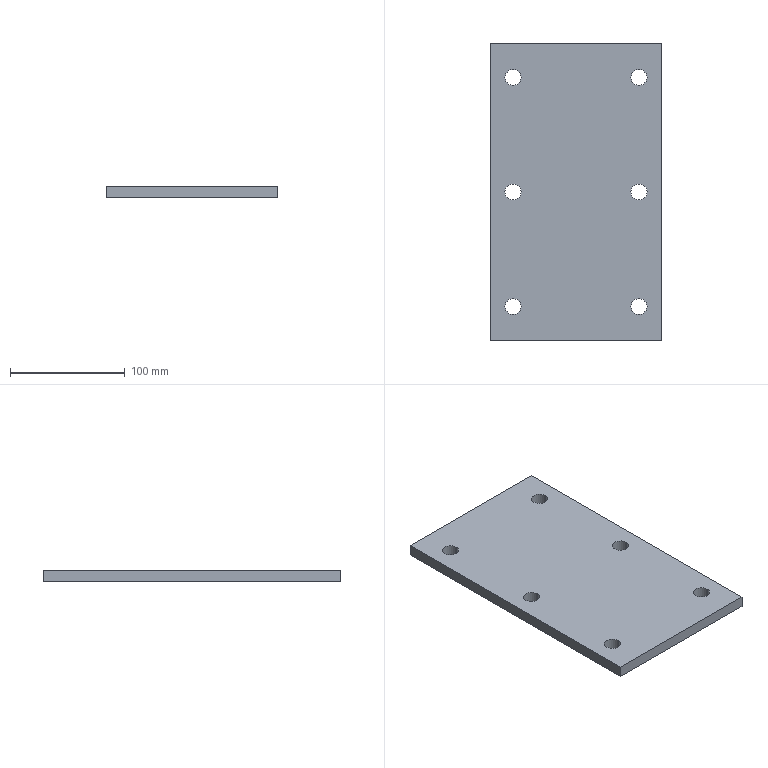Part | SolidWorks | features Extrusion 1, HoleWzd 1 | 1 solid | 18 faces | box 150 x 260 x 10 mm | volume 380764 mm3 | cylinder 12 | plane 6 | commonest cylinder face diameters 14 x12
STEP:
#1=CARTESIAN_POINT('',(-62.,100.,0.));
#2=VERTEX_POINT('',#1);
#3=CARTESIAN_POINT('',(-48.,100.,0.));
#4=VERTEX_POINT('',#3);
#5=CARTESIAN_POINT('',(-55.,100.,0.));
#6=DIRECTION('',(0.,0.,1.));
#7=DIRECTION('',(1.,0.,0.));
#8=AXIS2_PLACEMENT_3D('',#5,#6,#7);
#9=CIRCLE('',#8,7.);
#10=EDGE_CURVE('',#2,#4,#9,.T.);
#11=ORIENTED_EDGE('',*,*,#10,.F.);
#12=CARTESIAN_POINT('',(-62.,100.,10.));
#13=VERTEX_POINT('',#12);
#14=CARTESIAN_POINT('',(-62.,100.,10.));
#15=DIRECTION('',(0.,0.,1.));
#16=VECTOR('',#15,1000.);
#17=LINE('',#14,#16);
#18=EDGE_CURVE('',#2,#13,#17,.T.);
#19=ORIENTED_EDGE('',*,*,#18,.T.);
#20=CARTESIAN_POINT('',(-48.,100.,10.));
#21=VERTEX_POINT('',#20);
#22=CARTESIAN_POINT('',(-55.,100.,10.));
#23=DIRECTION('',(0.,0.,1.));
#24=DIRECTION('',(1.,0.,0.));
#25=AXIS2_PLACEMENT_3D('',#22,#23,#24);
#26=CIRCLE('',#25,7.);
#27=EDGE_CURVE('',#13,#21,#26,.T.);
#28=ORIENTED_EDGE('',*,*,#27,.T.);
#29=CARTESIAN_POINT('',(-48.,100.,10.));
#30=DIRECTION('',(0.,0.,1.));
#31=VECTOR('',#30,1000.);
#32=LINE('',#29,#31);
#33=EDGE_CURVE('',#4,#21,#32,.T.);
#34=ORIENTED_EDGE('',*,*,#33,.F.);
#35=EDGE_LOOP('',(#11,#19,#28,#34));
#36=FACE_OUTER_BOUND('',#35,.T.);
#37=CARTESIAN_POINT('',(-55.,100.,10.));
#38=DIRECTION('',(0.,0.,1.));
#39=DIRECTION('',(1.,0.,0.));
#40=AXIS2_PLACEMENT_3D('',#37,#38,#39);
#41=CYLINDRICAL_SURFACE('',#40,7.);
#42=ADVANCED_FACE('',(#36),#41,.F.);
#43=CARTESIAN_POINT('',(-62.,0.,0.));
#44=VERTEX_POINT('',#43);
#45=CARTESIAN_POINT('',(-48.,0.,0.));
#46=VERTEX_POINT('',#45);
#47=CARTESIAN_POINT('',(-55.,0.,0.));
#48=DIRECTION('',(0.,0.,1.));
#49=DIRECTION('',(1.,0.,0.));
#50=AXIS2_PLACEMENT_3D('',#47,#48,#49);
#51=CIRCLE('',#50,7.);
#52=EDGE_CURVE('',#44,#46,#51,.T.);
#53=ORIENTED_EDGE('',*,*,#52,.F.);
#54=CARTESIAN_POINT('',(-62.,0.,10.));
#55=VERTEX_POINT('',#54);
#56=CARTESIAN_POINT('',(-62.,0.,10.));
#57=DIRECTION('',(0.,0.,1.));
#58=VECTOR('',#57,1000.);
#59=LINE('',#56,#58);
#60=EDGE_CURVE('',#44,#55,#59,.T.);
#61=ORIENTED_EDGE('',*,*,#60,.T.);
#62=CARTESIAN_POINT('',(-48.,0.,10.));
#63=VERTEX_POINT('',#62);
#64=CARTESIAN_POINT('',(-55.,0.,10.));
#65=DIRECTION('',(0.,0.,1.));
#66=DIRECTION('',(1.,0.,0.));
#67=AXIS2_PLACEMENT_3D('',#64,#65,#66);
#68=CIRCLE('',#67,7.);
#69=EDGE_CURVE('',#55,#63,#68,.T.);
#70=ORIENTED_EDGE('',*,*,#69,.T.);
#71=CARTESIAN_POINT('',(-48.,0.,10.));
#72=DIRECTION('',(0.,0.,1.));
#73=VECTOR('',#72,1000.);
#74=LINE('',#71,#73);
#75=EDGE_CURVE('',#46,#63,#74,.T.);
#76=ORIENTED_EDGE('',*,*,#75,.F.);
#77=EDGE_LOOP('',(#53,#61,#70,#76));
#78=FACE_OUTER_BOUND('',#77,.T.);
#79=CARTESIAN_POINT('',(-55.,0.,10.));
#80=DIRECTION('',(0.,0.,1.));
#81=DIRECTION('',(1.,0.,0.));
#82=AXIS2_PLACEMENT_3D('',#79,#80,#81);
#83=CYLINDRICAL_SURFACE('',#82,7.);
#84=ADVANCED_FACE('',(#78),#83,.F.);
#85=CARTESIAN_POINT('',(-62.,-100.,0.));
#86=VERTEX_POINT('',#85);
#87=CARTESIAN_POINT('',(-48.,-100.,0.));
#88=VERTEX_POINT('',#87);
#89=CARTESIAN_POINT('',(-55.,-100.,0.));
#90=DIRECTION('',(0.,0.,1.));
#91=DIRECTION('',(1.,0.,0.));
#92=AXIS2_PLACEMENT_3D('',#89,#90,#91);
#93=CIRCLE('',#92,7.);
#94=EDGE_CURVE('',#86,#88,#93,.T.);
#95=ORIENTED_EDGE('',*,*,#94,.F.);
#96=CARTESIAN_POINT('',(-62.,-100.,10.));
#97=VERTEX_POINT('',#96);
#98=CARTESIAN_POINT('',(-62.,-100.,10.));
#99=DIRECTION('',(0.,0.,1.));
#100=VECTOR('',#99,1000.);
#101=LINE('',#98,#100);
#102=EDGE_CURVE('',#86,#97,#101,.T.);
#103=ORIENTED_EDGE('',*,*,#102,.T.);
#104=CARTESIAN_POINT('',(-48.,-100.,10.));
#105=VERTEX_POINT('',#104);
#106=CARTESIAN_POINT('',(-55.,-100.,10.));
#107=DIRECTION('',(0.,0.,1.));
#108=DIRECTION('',(1.,0.,0.));
#109=AXIS2_PLACEMENT_3D('',#106,#107,#108);
#110=CIRCLE('',#109,7.);
#111=EDGE_CURVE('',#97,#105,#110,.T.);
#112=ORIENTED_EDGE('',*,*,#111,.T.);
#113=CARTESIAN_POINT('',(-48.,-100.,10.));
#114=DIRECTION('',(0.,0.,1.));
#115=VECTOR('',#114,1000.);
#116=LINE('',#113,#115);
#117=EDGE_CURVE('',#88,#105,#116,.T.);
#118=ORIENTED_EDGE('',*,*,#117,.F.);
#119=EDGE_LOOP('',(#95,#103,#112,#118));
#120=FACE_OUTER_BOUND('',#119,.T.);
#121=CARTESIAN_POINT('',(-55.,-100.,10.));
#122=DIRECTION('',(0.,0.,1.));
#123=DIRECTION('',(1.,0.,0.));
#124=AXIS2_PLACEMENT_3D('',#121,#122,#123);
#125=CYLINDRICAL_SURFACE('',#124,7.);
#126=ADVANCED_FACE('',(#120),#125,.F.);
#127=CARTESIAN_POINT('',(48.,-100.,0.));
#128=VERTEX_POINT('',#127);
#129=CARTESIAN_POINT('',(62.,-100.,0.));
#130=VERTEX_POINT('',#129);
#131=CARTESIAN_POINT('',(55.,-100.,0.));
#132=DIRECTION('',(0.,0.,1.));
#133=DIRECTION('',(1.,0.,0.));
#134=AXIS2_PLACEMENT_3D('',#131,#132,#133);
#135=CIRCLE('',#134,7.);
#136=EDGE_CURVE('',#128,#130,#135,.T.);
#137=ORIENTED_EDGE('',*,*,#136,.F.);
#138=CARTESIAN_POINT('',(48.,-100.,10.));
#139=VERTEX_POINT('',#138);
#140=CARTESIAN_POINT('',(48.,-100.,10.));
#141=DIRECTION('',(0.,0.,1.));
#142=VECTOR('',#141,1000.);
#143=LINE('',#140,#142);
#144=EDGE_CURVE('',#128,#139,#143,.T.);
#145=ORIENTED_EDGE('',*,*,#144,.T.);
#146=CARTESIAN_POINT('',(62.,-100.,10.));
#147=VERTEX_POINT('',#146);
#148=CARTESIAN_POINT('',(55.,-100.,10.));
#149=DIRECTION('',(0.,0.,1.));
#150=DIRECTION('',(1.,0.,0.));
#151=AXIS2_PLACEMENT_3D('',#148,#149,#150);
#152=CIRCLE('',#151,7.);
#153=EDGE_CURVE('',#139,#147,#152,.T.);
#154=ORIENTED_EDGE('',*,*,#153,.T.);
#155=CARTESIAN_POINT('',(62.,-100.,10.));
#156=DIRECTION('',(0.,0.,1.));
#157=VECTOR('',#156,1000.);
#158=LINE('',#155,#157);
#159=EDGE_CURVE('',#130,#147,#158,.T.);
#160=ORIENTED_EDGE('',*,*,#159,.F.);
#161=EDGE_LOOP('',(#137,#145,#154,#160));
#162=FACE_OUTER_BOUND('',#161,.T.);
#163=CARTESIAN_POINT('',(55.,-100.,10.));
#164=DIRECTION('',(0.,0.,1.));
#165=DIRECTION('',(1.,0.,0.));
#166=AXIS2_PLACEMENT_3D('',#163,#164,#165);
#167=CYLINDRICAL_SURFACE('',#166,7.);
#168=ADVANCED_FACE('',(#162),#167,.F.);
#169=CARTESIAN_POINT('',(48.,0.,0.));
#170=VERTEX_POINT('',#169);
#171=CARTESIAN_POINT('',(62.,0.,0.));
#172=VERTEX_POINT('',#171);
#173=CARTESIAN_POINT('',(55.,0.,0.));
#174=DIRECTION('',(0.,0.,1.));
#175=DIRECTION('',(1.,0.,0.));
#176=AXIS2_PLACEMENT_3D('',#173,#174,#175);
#177=CIRCLE('',#176,7.);
#178=EDGE_CURVE('',#170,#172,#177,.T.);
#179=ORIENTED_EDGE('',*,*,#178,.F.);
#180=CARTESIAN_POINT('',(48.,0.,10.));
#181=VERTEX_POINT('',#180);
#182=CARTESIAN_POINT('',(48.,0.,10.));
#183=DIRECTION('',(0.,0.,1.));
#184=VECTOR('',#183,1000.);
#185=LINE('',#182,#184);
#186=EDGE_CURVE('',#170,#181,#185,.T.);
#187=ORIENTED_EDGE('',*,*,#186,.T.);
#188=CARTESIAN_POINT('',(62.,0.,10.));
#189=VERTEX_POINT('',#188);
#190=CARTESIAN_POINT('',(55.,0.,10.));
#191=DIRECTION('',(0.,0.,1.));
#192=DIRECTION('',(1.,0.,0.));
#193=AXIS2_PLACEMENT_3D('',#190,#191,#192);
#194=CIRCLE('',#193,7.);
#195=EDGE_CURVE('',#181,#189,#194,.T.);
#196=ORIENTED_EDGE('',*,*,#195,.T.);
#197=CARTESIAN_POINT('',(62.,0.,10.));
#198=DIRECTION('',(0.,0.,1.));
#199=VECTOR('',#198,1000.);
#200=LINE('',#197,#199);
#201=EDGE_CURVE('',#172,#189,#200,.T.);
#202=ORIENTED_EDGE('',*,*,#201,.F.);
#203=EDGE_LOOP('',(#179,#187,#196,#202));
#204=FACE_OUTER_BOUND('',#203,.T.);
#205=CARTESIAN_POINT('',(55.,0.,10.));
#206=DIRECTION('',(0.,0.,1.));
#207=DIRECTION('',(1.,0.,0.));
#208=AXIS2_PLACEMENT_3D('',#205,#206,#207);
#209=CYLINDRICAL_SURFACE('',#208,7.);
#210=ADVANCED_FACE('',(#204),#209,.F.);
#211=CARTESIAN_POINT('',(48.,100.,0.));
#212=VERTEX_POINT('',#211);
#213=CARTESIAN_POINT('',(62.,100.,0.));
#214=VERTEX_POINT('',#213);
#215=CARTESIAN_POINT('',(55.,100.,0.));
#216=DIRECTION('',(0.,0.,1.));
#217=DIRECTION('',(1.,0.,0.));
#218=AXIS2_PLACEMENT_3D('',#215,#216,#217);
#219=CIRCLE('',#218,7.);
#220=EDGE_CURVE('',#212,#214,#219,.T.);
#221=ORIENTED_EDGE('',*,*,#220,.F.);
#222=CARTESIAN_POINT('',(48.,100.,10.));
#223=VERTEX_POINT('',#222);
#224=CARTESIAN_POINT('',(48.,100.,10.));
#225=DIRECTION('',(0.,0.,1.));
#226=VECTOR('',#225,1000.);
#227=LINE('',#224,#226);
#228=EDGE_CURVE('',#212,#223,#227,.T.);
#229=ORIENTED_EDGE('',*,*,#228,.T.);
#230=CARTESIAN_POINT('',(62.,100.,10.));
#231=VERTEX_POINT('',#230);
#232=CARTESIAN_POINT('',(55.,100.,10.));
#233=DIRECTION('',(0.,0.,1.));
#234=DIRECTION('',(1.,0.,0.));
#235=AXIS2_PLACEMENT_3D('',#232,#233,#234);
#236=CIRCLE('',#235,7.);
#237=EDGE_CURVE('',#223,#231,#236,.T.);
#238=ORIENTED_EDGE('',*,*,#237,.T.);
#239=CARTESIAN_POINT('',(62.,100.,10.));
#240=DIRECTION('',(0.,0.,1.));
#241=VECTOR('',#240,1000.);
#242=LINE('',#239,#241);
#243=EDGE_CURVE('',#214,#231,#242,.T.);
#244=ORIENTED_EDGE('',*,*,#243,.F.);
#245=EDGE_LOOP('',(#221,#229,#238,#244));
#246=FACE_OUTER_BOUND('',#245,.T.);
#247=CARTESIAN_POINT('',(55.,100.,10.));
#248=DIRECTION('',(0.,0.,1.));
#249=DIRECTION('',(1.,0.,0.));
#250=AXIS2_PLACEMENT_3D('',#247,#248,#249);
#251=CYLINDRICAL_SURFACE('',#250,7.);
#252=ADVANCED_FACE('',(#246),#251,.F.);
#253=CARTESIAN_POINT('',(-75.,130.,0.));
#254=VERTEX_POINT('',#253);
#255=CARTESIAN_POINT('',(-75.,-130.,0.));
#256=VERTEX_POINT('',#255);
#257=CARTESIAN_POINT('',(-75.,-130.,0.));
#258=DIRECTION('',(0.,-1.,0.));
#259=VECTOR('',#258,1000.);
#260=LINE('',#257,#259);
#261=EDGE_CURVE('',#254,#256,#260,.T.);
#262=ORIENTED_EDGE('',*,*,#261,.T.);
#263=CARTESIAN_POINT('',(-75.,-130.,10.));
#264=VERTEX_POINT('',#263);
#265=CARTESIAN_POINT('',(-75.,-130.,10.));
#266=DIRECTION('',(0.,0.,-1.));
#267=VECTOR('',#266,1000.);
#268=LINE('',#265,#267);
#269=EDGE_CURVE('',#264,#256,#268,.T.);
#270=ORIENTED_EDGE('',*,*,#269,.F.);
#271=CARTESIAN_POINT('',(-75.,130.,10.));
#272=VERTEX_POINT('',#271);
#273=CARTESIAN_POINT('',(-75.,-130.,10.));
#274=DIRECTION('',(0.,-1.,0.));
#275=VECTOR('',#274,1000.);
#276=LINE('',#273,#275);
#277=EDGE_CURVE('',#272,#264,#276,.T.);
#278=ORIENTED_EDGE('',*,*,#277,.F.);
#279=CARTESIAN_POINT('',(-75.,130.,10.));
#280=DIRECTION('',(0.,0.,-1.));
#281=VECTOR('',#280,1000.);
#282=LINE('',#279,#281);
#283=EDGE_CURVE('',#272,#254,#282,.T.);
#284=ORIENTED_EDGE('',*,*,#283,.T.);
#285=EDGE_LOOP('',(#262,#270,#278,#284));
#286=FACE_OUTER_BOUND('',#285,.T.);
#287=CARTESIAN_POINT('',(-75.,-130.,10.));
#288=DIRECTION('',(1.,0.,0.));
#289=DIRECTION('',(0.,0.,-1.));
#290=AXIS2_PLACEMENT_3D('',#287,#288,#289);
#291=PLANE('',#290);
#292=ADVANCED_FACE('',(#286),#291,.F.);
#293=CARTESIAN_POINT('',(75.,-130.,0.));
#294=VERTEX_POINT('',#293);
#295=CARTESIAN_POINT('',(75.,-130.,0.));
#296=DIRECTION('',(1.,0.,0.));
#297=VECTOR('',#296,1000.);
#298=LINE('',#295,#297);
#299=EDGE_CURVE('',#256,#294,#298,.T.);
#300=ORIENTED_EDGE('',*,*,#299,.T.);
#301=CARTESIAN_POINT('',(75.,-130.,10.));
#302=VERTEX_POINT('',#301);
#303=CARTESIAN_POINT('',(75.,-130.,10.));
#304=DIRECTION('',(0.,0.,-1.));
#305=VECTOR('',#304,1000.);
#306=LINE('',#303,#305);
#307=EDGE_CURVE('',#302,#294,#306,.T.);
#308=ORIENTED_EDGE('',*,*,#307,.F.);
#309=CARTESIAN_POINT('',(75.,-130.,10.));
#310=DIRECTION('',(1.,0.,0.));
#311=VECTOR('',#310,1000.);
#312=LINE('',#309,#311);
#313=EDGE_CURVE('',#264,#302,#312,.T.);
#314=ORIENTED_EDGE('',*,*,#313,.F.);
#315=ORIENTED_EDGE('',*,*,#269,.T.);
#316=EDGE_LOOP('',(#300,#308,#314,#315));
#317=FACE_OUTER_BOUND('',#316,.T.);
#318=CARTESIAN_POINT('',(75.,-130.,10.));
#319=DIRECTION('',(0.,1.,0.));
#320=DIRECTION('',(-1.,0.,0.));
#321=AXIS2_PLACEMENT_3D('',#318,#319,#320);
#322=PLANE('',#321);
#323=ADVANCED_FACE('',(#317),#322,.F.);
#324=CARTESIAN_POINT('',(75.,130.,0.));
#325=VERTEX_POINT('',#324);
#326=CARTESIAN_POINT('',(75.,-130.,0.));
#327=DIRECTION('',(0.,1.,0.));
#328=VECTOR('',#327,1000.);
#329=LINE('',#326,#328);
#330=EDGE_CURVE('',#294,#325,#329,.T.);
#331=ORIENTED_EDGE('',*,*,#330,.T.);
#332=CARTESIAN_POINT('',(75.,130.,10.));
#333=VERTEX_POINT('',#332);
#334=CARTESIAN_POINT('',(75.,130.,10.));
#335=DIRECTION('',(0.,0.,-1.));
#336=VECTOR('',#335,1000.);
#337=LINE('',#334,#336);
#338=EDGE_CURVE('',#333,#325,#337,.T.);
#339=ORIENTED_EDGE('',*,*,#338,.F.);
#340=CARTESIAN_POINT('',(75.,-130.,10.));
#341=DIRECTION('',(0.,1.,0.));
#342=VECTOR('',#341,1000.);
#343=LINE('',#340,#342);
#344=EDGE_CURVE('',#302,#333,#343,.T.);
#345=ORIENTED_EDGE('',*,*,#344,.F.);
#346=ORIENTED_EDGE('',*,*,#307,.T.);
#347=EDGE_LOOP('',(#331,#339,#345,#346));
#348=FACE_OUTER_BOUND('',#347,.T.);
#349=CARTESIAN_POINT('',(75.,-130.,10.));
#350=DIRECTION('',(-1.,0.,0.));
#351=DIRECTION('',(0.,0.,1.));
#352=AXIS2_PLACEMENT_3D('',#349,#350,#351);
#353=PLANE('',#352);
#354=ADVANCED_FACE('',(#348),#353,.F.);
#355=CARTESIAN_POINT('',(75.,130.,0.));
#356=DIRECTION('',(-1.,0.,0.));
#357=VECTOR('',#356,1000.);
#358=LINE('',#355,#357);
#359=EDGE_CURVE('',#325,#254,#358,.T.);
#360=ORIENTED_EDGE('',*,*,#359,.T.);
#361=ORIENTED_EDGE('',*,*,#283,.F.);
#362=CARTESIAN_POINT('',(75.,130.,10.));
#363=DIRECTION('',(-1.,0.,0.));
#364=VECTOR('',#363,1000.);
#365=LINE('',#362,#364);
#366=EDGE_CURVE('',#333,#272,#365,.T.);
#367=ORIENTED_EDGE('',*,*,#366,.F.);
#368=ORIENTED_EDGE('',*,*,#338,.T.);
#369=EDGE_LOOP('',(#360,#361,#367,#368));
#370=FACE_OUTER_BOUND('',#369,.T.);
#371=CARTESIAN_POINT('',(75.,130.,10.));
#372=DIRECTION('',(0.,-1.,0.));
#373=DIRECTION('',(0.,0.,-1.));
#374=AXIS2_PLACEMENT_3D('',#371,#372,#373);
#375=PLANE('',#374);
#376=ADVANCED_FACE('',(#370),#375,.F.);
#377=CARTESIAN_POINT('',(-55.,100.,10.));
#378=DIRECTION('',(0.,0.,1.));
#379=DIRECTION('',(1.,0.,0.));
#380=AXIS2_PLACEMENT_3D('',#377,#378,#379);
#381=CIRCLE('',#380,7.);
#382=EDGE_CURVE('',#21,#13,#381,.T.);
#383=ORIENTED_EDGE('',*,*,#382,.F.);
#384=ORIENTED_EDGE('',*,*,#27,.F.);
#385=EDGE_LOOP('',(#383,#384));
#386=FACE_BOUND('',#385,.T.);
#387=CARTESIAN_POINT('',(-55.,0.,10.));
#388=DIRECTION('',(0.,0.,1.));
#389=DIRECTION('',(1.,0.,0.));
#390=AXIS2_PLACEMENT_3D('',#387,#388,#389);
#391=CIRCLE('',#390,7.);
#392=EDGE_CURVE('',#63,#55,#391,.T.);
#393=ORIENTED_EDGE('',*,*,#392,.F.);
#394=ORIENTED_EDGE('',*,*,#69,.F.);
#395=EDGE_LOOP('',(#393,#394));
#396=FACE_BOUND('',#395,.T.);
#397=CARTESIAN_POINT('',(-55.,-100.,10.));
#398=DIRECTION('',(0.,0.,1.));
#399=DIRECTION('',(1.,0.,0.));
#400=AXIS2_PLACEMENT_3D('',#397,#398,#399);
#401=CIRCLE('',#400,7.);
#402=EDGE_CURVE('',#105,#97,#401,.T.);
#403=ORIENTED_EDGE('',*,*,#402,.F.);
#404=ORIENTED_EDGE('',*,*,#111,.F.);
#405=EDGE_LOOP('',(#403,#404));
#406=FACE_BOUND('',#405,.T.);
#407=CARTESIAN_POINT('',(55.,-100.,10.));
#408=DIRECTION('',(0.,0.,1.));
#409=DIRECTION('',(1.,0.,0.));
#410=AXIS2_PLACEMENT_3D('',#407,#408,#409);
#411=CIRCLE('',#410,7.);
#412=EDGE_CURVE('',#147,#139,#411,.T.);
#413=ORIENTED_EDGE('',*,*,#412,.F.);
#414=ORIENTED_EDGE('',*,*,#153,.F.);
#415=EDGE_LOOP('',(#413,#414));
#416=FACE_BOUND('',#415,.T.);
#417=CARTESIAN_POINT('',(55.,0.,10.));
#418=DIRECTION('',(0.,0.,1.));
#419=DIRECTION('',(1.,0.,0.));
#420=AXIS2_PLACEMENT_3D('',#417,#418,#419);
#421=CIRCLE('',#420,7.);
#422=EDGE_CURVE('',#189,#181,#421,.T.);
#423=ORIENTED_EDGE('',*,*,#422,.F.);
#424=ORIENTED_EDGE('',*,*,#195,.F.);
#425=EDGE_LOOP('',(#423,#424));
#426=FACE_BOUND('',#425,.T.);
#427=CARTESIAN_POINT('',(55.,100.,10.));
#428=DIRECTION('',(0.,0.,1.));
#429=DIRECTION('',(1.,0.,0.));
#430=AXIS2_PLACEMENT_3D('',#427,#428,#429);
#431=CIRCLE('',#430,7.);
#432=EDGE_CURVE('',#231,#223,#431,.T.);
#433=ORIENTED_EDGE('',*,*,#432,.F.);
#434=ORIENTED_EDGE('',*,*,#237,.F.);
#435=EDGE_LOOP('',(#433,#434));
#436=FACE_BOUND('',#435,.T.);
#437=ORIENTED_EDGE('',*,*,#277,.T.);
#438=ORIENTED_EDGE('',*,*,#313,.T.);
#439=ORIENTED_EDGE('',*,*,#344,.T.);
#440=ORIENTED_EDGE('',*,*,#366,.T.);
#441=EDGE_LOOP('',(#437,#438,#439,#440));
#442=FACE_OUTER_BOUND('',#441,.T.);
#443=CARTESIAN_POINT('',(0.,0.,10.));
#444=DIRECTION('',(0.,0.,1.));
#445=DIRECTION('',(1.,0.,0.));
#446=AXIS2_PLACEMENT_3D('',#443,#444,#445);
#447=PLANE('',#446);
#448=ADVANCED_FACE('',(#386,#396,#406,#416,#426,#436,#442),#447,.T.);
#449=CARTESIAN_POINT('',(-55.,100.,0.));
#450=DIRECTION('',(0.,0.,1.));
#451=DIRECTION('',(1.,0.,0.));
#452=AXIS2_PLACEMENT_3D('',#449,#450,#451);
#453=CIRCLE('',#452,7.);
#454=EDGE_CURVE('',#4,#2,#453,.T.);
#455=ORIENTED_EDGE('',*,*,#454,.T.);
#456=ORIENTED_EDGE('',*,*,#10,.T.);
#457=EDGE_LOOP('',(#455,#456));
#458=FACE_BOUND('',#457,.T.);
#459=CARTESIAN_POINT('',(-55.,0.,0.));
#460=DIRECTION('',(0.,0.,1.));
#461=DIRECTION('',(1.,0.,0.));
#462=AXIS2_PLACEMENT_3D('',#459,#460,#461);
#463=CIRCLE('',#462,7.);
#464=EDGE_CURVE('',#46,#44,#463,.T.);
#465=ORIENTED_EDGE('',*,*,#464,.T.);
#466=ORIENTED_EDGE('',*,*,#52,.T.);
#467=EDGE_LOOP('',(#465,#466));
#468=FACE_BOUND('',#467,.T.);
#469=CARTESIAN_POINT('',(-55.,-100.,0.));
#470=DIRECTION('',(0.,0.,1.));
#471=DIRECTION('',(1.,0.,0.));
#472=AXIS2_PLACEMENT_3D('',#469,#470,#471);
#473=CIRCLE('',#472,7.);
#474=EDGE_CURVE('',#88,#86,#473,.T.);
#475=ORIENTED_EDGE('',*,*,#474,.T.);
#476=ORIENTED_EDGE('',*,*,#94,.T.);
#477=EDGE_LOOP('',(#475,#476));
#478=FACE_BOUND('',#477,.T.);
#479=CARTESIAN_POINT('',(55.,-100.,0.));
#480=DIRECTION('',(0.,0.,1.));
#481=DIRECTION('',(1.,0.,0.));
#482=AXIS2_PLACEMENT_3D('',#479,#480,#481);
#483=CIRCLE('',#482,7.);
#484=EDGE_CURVE('',#130,#128,#483,.T.);
#485=ORIENTED_EDGE('',*,*,#484,.T.);
#486=ORIENTED_EDGE('',*,*,#136,.T.);
#487=EDGE_LOOP('',(#485,#486));
#488=FACE_BOUND('',#487,.T.);
#489=CARTESIAN_POINT('',(55.,0.,0.));
#490=DIRECTION('',(0.,0.,1.));
#491=DIRECTION('',(1.,0.,0.));
#492=AXIS2_PLACEMENT_3D('',#489,#490,#491);
#493=CIRCLE('',#492,7.);
#494=EDGE_CURVE('',#172,#170,#493,.T.);
#495=ORIENTED_EDGE('',*,*,#494,.T.);
#496=ORIENTED_EDGE('',*,*,#178,.T.);
#497=EDGE_LOOP('',(#495,#496));
#498=FACE_BOUND('',#497,.T.);
#499=CARTESIAN_POINT('',(55.,100.,0.));
#500=DIRECTION('',(0.,0.,1.));
#501=DIRECTION('',(1.,0.,0.));
#502=AXIS2_PLACEMENT_3D('',#499,#500,#501);
#503=CIRCLE('',#502,7.);
#504=EDGE_CURVE('',#214,#212,#503,.T.);
#505=ORIENTED_EDGE('',*,*,#504,.T.);
#506=ORIENTED_EDGE('',*,*,#220,.T.);
#507=EDGE_LOOP('',(#505,#506));
#508=FACE_BOUND('',#507,.T.);
#509=ORIENTED_EDGE('',*,*,#261,.F.);
#510=ORIENTED_EDGE('',*,*,#359,.F.);
#511=ORIENTED_EDGE('',*,*,#330,.F.);
#512=ORIENTED_EDGE('',*,*,#299,.F.);
#513=EDGE_LOOP('',(#509,#510,#511,#512));
#514=FACE_OUTER_BOUND('',#513,.T.);
#515=CARTESIAN_POINT('',(0.,0.,0.));
#516=DIRECTION('',(0.,0.,1.));
#517=DIRECTION('',(1.,0.,0.));
#518=AXIS2_PLACEMENT_3D('',#515,#516,#517);
#519=PLANE('',#518);
#520=ADVANCED_FACE('',(#458,#468,#478,#488,#498,#508,#514),#519,.F.);
#521=ORIENTED_EDGE('',*,*,#228,.F.);
#522=ORIENTED_EDGE('',*,*,#504,.F.);
#523=ORIENTED_EDGE('',*,*,#243,.T.);
#524=ORIENTED_EDGE('',*,*,#432,.T.);
#525=EDGE_LOOP('',(#521,#522,#523,#524));
#526=FACE_OUTER_BOUND('',#525,.T.);
#527=CARTESIAN_POINT('',(55.,100.,10.));
#528=DIRECTION('',(0.,0.,1.));
#529=DIRECTION('',(1.,0.,0.));
#530=AXIS2_PLACEMENT_3D('',#527,#528,#529);
#531=CYLINDRICAL_SURFACE('',#530,7.);
#532=ADVANCED_FACE('',(#526),#531,.F.);
#533=ORIENTED_EDGE('',*,*,#186,.F.);
#534=ORIENTED_EDGE('',*,*,#494,.F.);
#535=ORIENTED_EDGE('',*,*,#201,.T.);
#536=ORIENTED_EDGE('',*,*,#422,.T.);
#537=EDGE_LOOP('',(#533,#534,#535,#536));
#538=FACE_OUTER_BOUND('',#537,.T.);
#539=CARTESIAN_POINT('',(55.,0.,10.));
#540=DIRECTION('',(0.,0.,1.));
#541=DIRECTION('',(1.,0.,0.));
#542=AXIS2_PLACEMENT_3D('',#539,#540,#541);
#543=CYLINDRICAL_SURFACE('',#542,7.);
#544=ADVANCED_FACE('',(#538),#543,.F.);
#545=ORIENTED_EDGE('',*,*,#144,.F.);
#546=ORIENTED_EDGE('',*,*,#484,.F.);
#547=ORIENTED_EDGE('',*,*,#159,.T.);
#548=ORIENTED_EDGE('',*,*,#412,.T.);
#549=EDGE_LOOP('',(#545,#546,#547,#548));
#550=FACE_OUTER_BOUND('',#549,.T.);
#551=CARTESIAN_POINT('',(55.,-100.,10.));
#552=DIRECTION('',(0.,0.,1.));
#553=DIRECTION('',(1.,0.,0.));
#554=AXIS2_PLACEMENT_3D('',#551,#552,#553);
#555=CYLINDRICAL_SURFACE('',#554,7.);
#556=ADVANCED_FACE('',(#550),#555,.F.);
#557=ORIENTED_EDGE('',*,*,#102,.F.);
#558=ORIENTED_EDGE('',*,*,#474,.F.);
#559=ORIENTED_EDGE('',*,*,#117,.T.);
#560=ORIENTED_EDGE('',*,*,#402,.T.);
#561=EDGE_LOOP('',(#557,#558,#559,#560));
#562=FACE_OUTER_BOUND('',#561,.T.);
#563=CARTESIAN_POINT('',(-55.,-100.,10.));
#564=DIRECTION('',(0.,0.,1.));
#565=DIRECTION('',(1.,0.,0.));
#566=AXIS2_PLACEMENT_3D('',#563,#564,#565);
#567=CYLINDRICAL_SURFACE('',#566,7.);
#568=ADVANCED_FACE('',(#562),#567,.F.);
#569=ORIENTED_EDGE('',*,*,#60,.F.);
#570=ORIENTED_EDGE('',*,*,#464,.F.);
#571=ORIENTED_EDGE('',*,*,#75,.T.);
#572=ORIENTED_EDGE('',*,*,#392,.T.);
#573=EDGE_LOOP('',(#569,#570,#571,#572));
#574=FACE_OUTER_BOUND('',#573,.T.);
#575=CARTESIAN_POINT('',(-55.,0.,10.));
#576=DIRECTION('',(0.,0.,1.));
#577=DIRECTION('',(1.,0.,0.));
#578=AXIS2_PLACEMENT_3D('',#575,#576,#577);
#579=CYLINDRICAL_SURFACE('',#578,7.);
#580=ADVANCED_FACE('',(#574),#579,.F.);
#581=ORIENTED_EDGE('',*,*,#18,.F.);
#582=ORIENTED_EDGE('',*,*,#454,.F.);
#583=ORIENTED_EDGE('',*,*,#33,.T.);
#584=ORIENTED_EDGE('',*,*,#382,.T.);
#585=EDGE_LOOP('',(#581,#582,#583,#584));
#586=FACE_OUTER_BOUND('',#585,.T.);
#587=CARTESIAN_POINT('',(-55.,100.,10.));
#588=DIRECTION('',(0.,0.,1.));
#589=DIRECTION('',(1.,0.,0.));
#590=AXIS2_PLACEMENT_3D('',#587,#588,#589);
#591=CYLINDRICAL_SURFACE('',#590,7.);
#592=ADVANCED_FACE('',(#586),#591,.F.);
#593=CLOSED_SHELL('',(#42,#84,#126,#168,#210,#252,#292,#323,#354,#376,#448,#520,#532,#544,#556,#568,#580,#592));
#594=MANIFOLD_SOLID_BREP('',#593);
#595=CARTESIAN_POINT('',(0.,0.,0.));
#596=DIRECTION('',(0.,0.,1.));
#597=DIRECTION('',(1.,0.,0.));
#598=AXIS2_PLACEMENT_3D('',#595,#596,#597);
#599=(LENGTH_UNIT()NAMED_UNIT(*)SI_UNIT(.MILLI.,.METRE.));
#600=UNCERTAINTY_MEASURE_WITH_UNIT(LENGTH_MEASURE(0.00001),#599,'','');
#601=(NAMED_UNIT(*)PLANE_ANGLE_UNIT()SI_UNIT($,.RADIAN.));
#602=(NAMED_UNIT(*)SI_UNIT($,.STERADIAN.)SOLID_ANGLE_UNIT());
#603=(GEOMETRIC_REPRESENTATION_CONTEXT(3)GLOBAL_UNCERTAINTY_ASSIGNED_CONTEXT((#600))GLOBAL_UNIT_ASSIGNED_CONTEXT((#599,#601,#602))REPRESENTATION_CONTEXT('',''));
#604=ADVANCED_BREP_SHAPE_REPRESENTATION('',(#594,#598),#603);